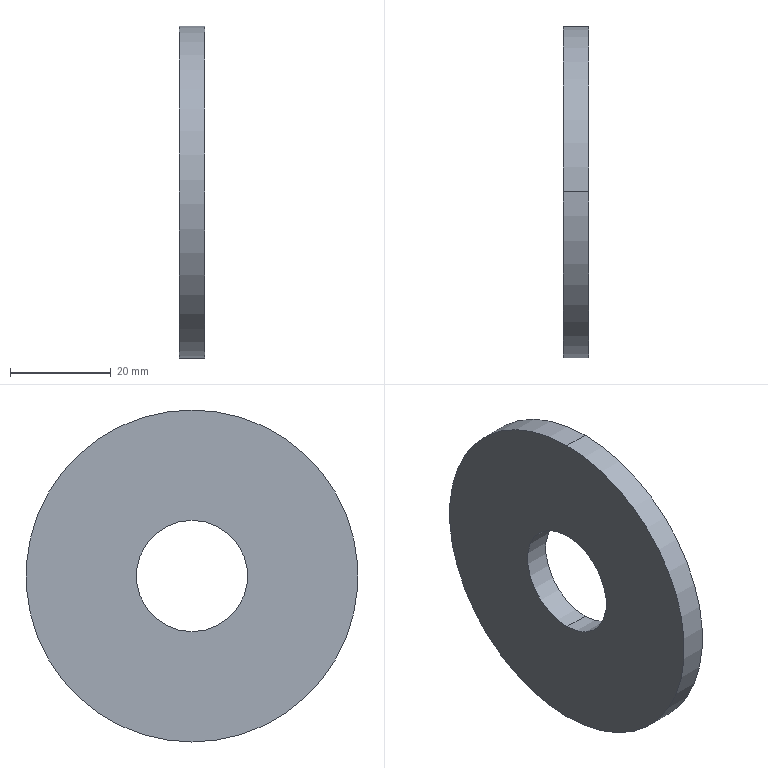Part | STEP file | flat washer wide_am_B18.22M - Plain washer, 20 mm, wide | 1 solid | 6 faces | box 5.1 x 66 x 66 mm | volume 15486 mm3 | cylinder 4 | plane 2 | commonest cylinder face diameters 22.13 x2 66 x2
STEP:
#1=CARTESIAN_POINT('',(0.,0.,0.));
#2=DIRECTION('',(0.,0.,1.));
#3=DIRECTION('',(1.,0.,0.));
#4=AXIS2_PLACEMENT_3D('',#1,#2,#3);
#5=CARTESIAN_POINT('',(0.,0.,33.));
#6=VERTEX_POINT('',#5);
#7=CARTESIAN_POINT('',(0.,0.,-33.));
#8=VERTEX_POINT('',#7);
#9=CARTESIAN_POINT('',(0.,0.,0.));
#10=DIRECTION('',(-1.,0.,0.));
#11=DIRECTION('',(0.,0.,1.));
#12=AXIS2_PLACEMENT_3D('',#9,#10,#11);
#13=CIRCLE('',#12,33.);
#14=CARTESIAN_POINT('',(-34.925,0.,0.));
#15=DIRECTION('',(-1.,0.,0.));
#16=DIRECTION('',(0.,0.,1.));
#17=AXIS2_PLACEMENT_3D('',#14,#15,#16);
#18=CYLINDRICAL_SURFACE('',#17,33.);
#19=CARTESIAN_POINT('',(0.,-34.925));
#20=DIRECTION('',(1.,0.));
#21=VECTOR('',#20,1.);
#22=LINE('',#19,#21);
#23=(GEOMETRIC_REPRESENTATION_CONTEXT(2)PARAMETRIC_REPRESENTATION_CONTEXT()REPRESENTATION_CONTEXT('',''));
#24=DEFINITIONAL_REPRESENTATION('',(#22),#23);
#25=PCURVE('',#18,#24);
#26=CARTESIAN_POINT('',(0.,11.065,0.));
#27=DIRECTION('',(-1.,0.,0.));
#28=DIRECTION('',(0.,0.,1.));
#29=AXIS2_PLACEMENT_3D('',#26,#27,#28);
#30=PLANE('',#29);
#31=CARTESIAN_POINT('',(0.,-11.065));
#32=DIRECTION('',(1.,0.));
#33=AXIS2_PLACEMENT_2D('',#31,#32);
#34=CIRCLE('',#33,33.);
#35=(GEOMETRIC_REPRESENTATION_CONTEXT(2)PARAMETRIC_REPRESENTATION_CONTEXT()REPRESENTATION_CONTEXT('',''));
#36=DEFINITIONAL_REPRESENTATION('',(#34),#35);
#37=PCURVE('',#30,#36);
#38=SURFACE_CURVE('',#13,(#25,#37),.PCURVE_S1.);
#39=EDGE_CURVE('',#6,#8,#38,.T.);
#40=ORIENTED_EDGE('',*,*,#39,.T.);
#41=CARTESIAN_POINT('',(-5.1,0.,-33.));
#42=VERTEX_POINT('',#41);
#43=CARTESIAN_POINT('',(-34.925,0.,-33.));
#44=DIRECTION('',(-1.,0.,0.));
#45=VECTOR('',#44,1.);
#46=LINE('',#43,#45);
#47=CARTESIAN_POINT('',(3.142,0.));
#48=DIRECTION('',(0.,1.));
#49=VECTOR('',#48,1.);
#50=LINE('',#47,#49);
#51=(GEOMETRIC_REPRESENTATION_CONTEXT(2)PARAMETRIC_REPRESENTATION_CONTEXT()REPRESENTATION_CONTEXT('',''));
#52=DEFINITIONAL_REPRESENTATION('',(#50),#51);
#53=PCURVE('',#18,#52);
#54=CARTESIAN_POINT('',(-34.925,0.,0.));
#55=DIRECTION('',(-1.,0.,0.));
#56=DIRECTION('',(0.,0.,1.));
#57=AXIS2_PLACEMENT_3D('',#54,#55,#56);
#58=CYLINDRICAL_SURFACE('',#57,33.);
#59=CARTESIAN_POINT('',(3.142,0.));
#60=DIRECTION('',(0.,1.));
#61=VECTOR('',#60,1.);
#62=LINE('',#59,#61);
#63=(GEOMETRIC_REPRESENTATION_CONTEXT(2)PARAMETRIC_REPRESENTATION_CONTEXT()REPRESENTATION_CONTEXT('',''));
#64=DEFINITIONAL_REPRESENTATION('',(#62),#63);
#65=PCURVE('',#58,#64);
#66=SURFACE_CURVE('',#46,(#53,#65),.PCURVE_S1.);
#67=EDGE_CURVE('',#8,#42,#66,.T.);
#68=ORIENTED_EDGE('',*,*,#67,.T.);
#69=CARTESIAN_POINT('',(-5.1,0.,33.));
#70=VERTEX_POINT('',#69);
#71=CARTESIAN_POINT('',(-5.1,0.,0.));
#72=DIRECTION('',(-1.,0.,0.));
#73=DIRECTION('',(0.,0.,1.));
#74=AXIS2_PLACEMENT_3D('',#71,#72,#73);
#75=CIRCLE('',#74,33.);
#76=CARTESIAN_POINT('',(0.,-29.825));
#77=DIRECTION('',(1.,0.));
#78=VECTOR('',#77,1.);
#79=LINE('',#76,#78);
#80=(GEOMETRIC_REPRESENTATION_CONTEXT(2)PARAMETRIC_REPRESENTATION_CONTEXT()REPRESENTATION_CONTEXT('',''));
#81=DEFINITIONAL_REPRESENTATION('',(#79),#80);
#82=PCURVE('',#18,#81);
#83=CARTESIAN_POINT('',(-5.1,33.,0.));
#84=DIRECTION('',(1.,0.,0.));
#85=DIRECTION('',(0.,0.,-1.));
#86=AXIS2_PLACEMENT_3D('',#83,#84,#85);
#87=PLANE('',#86);
#88=CARTESIAN_POINT('',(-33.,-33.));
#89=CARTESIAN_POINT('',(-33.,24.158));
#90=CARTESIAN_POINT('',(16.5,-4.421));
#91=CARTESIAN_POINT('',(66.,-33.));
#92=CARTESIAN_POINT('',(16.5,-61.579));
#93=CARTESIAN_POINT('',(-33.,-90.158));
#94=CARTESIAN_POINT('',(-33.,-33.));
#95=(BOUNDED_CURVE()B_SPLINE_CURVE(2,(#88,#89,#90,#91,#92,#93,#94),.UNSPECIFIED.,.T.,.F.)B_SPLINE_CURVE_WITH_KNOTS((1,2,2,2,2,1),(-2.094,0.,2.094,4.189,6.283,8.378),.UNSPECIFIED.)CURVE()GEOMETRIC_REPRESENTATION_ITEM()RATIONAL_B_SPLINE_CURVE((1.,0.5,1.,0.5,1.,0.5,1.))REPRESENTATION_ITEM(''));
#96=(GEOMETRIC_REPRESENTATION_CONTEXT(2)PARAMETRIC_REPRESENTATION_CONTEXT()REPRESENTATION_CONTEXT('',''));
#97=DEFINITIONAL_REPRESENTATION('',(#95),#96);
#98=PCURVE('',#87,#97);
#99=SURFACE_CURVE('',#75,(#82,#98),.PCURVE_S1.);
#100=EDGE_CURVE('',#70,#42,#99,.T.);
#101=ORIENTED_EDGE('',*,*,#100,.F.);
#102=CARTESIAN_POINT('',(-34.925,0.,33.));
#103=DIRECTION('',(-1.,0.,0.));
#104=VECTOR('',#103,1.);
#105=LINE('',#102,#104);
#106=CARTESIAN_POINT('',(0.,0.));
#107=DIRECTION('',(0.,1.));
#108=VECTOR('',#107,1.);
#109=LINE('',#106,#108);
#110=(GEOMETRIC_REPRESENTATION_CONTEXT(2)PARAMETRIC_REPRESENTATION_CONTEXT()REPRESENTATION_CONTEXT('',''));
#111=DEFINITIONAL_REPRESENTATION('',(#109),#110);
#112=PCURVE('',#18,#111);
#113=CARTESIAN_POINT('',(6.283,0.));
#114=DIRECTION('',(0.,1.));
#115=VECTOR('',#114,1.);
#116=LINE('',#113,#115);
#117=(GEOMETRIC_REPRESENTATION_CONTEXT(2)PARAMETRIC_REPRESENTATION_CONTEXT()REPRESENTATION_CONTEXT('',''));
#118=DEFINITIONAL_REPRESENTATION('',(#116),#117);
#119=PCURVE('',#58,#118);
#120=SURFACE_CURVE('',#105,(#112,#119),.PCURVE_S1.);
#121=EDGE_CURVE('',#6,#70,#120,.T.);
#122=ORIENTED_EDGE('',*,*,#121,.F.);
#123=EDGE_LOOP('',(#40,#68,#101,#122));
#124=FACE_BOUND('',#123,.T.);
#125=ADVANCED_FACE('',(#124),#18,.T.);
#126=CARTESIAN_POINT('',(0.,0.,11.065));
#127=VERTEX_POINT('',#126);
#128=CARTESIAN_POINT('',(-5.1,0.,11.065));
#129=VERTEX_POINT('',#128);
#130=CARTESIAN_POINT('',(-34.925,0.,11.065));
#131=DIRECTION('',(-1.,0.,0.));
#132=VECTOR('',#131,1.);
#133=LINE('',#130,#132);
#134=CARTESIAN_POINT('',(-34.925,0.,0.));
#135=DIRECTION('',(-1.,0.,0.));
#136=DIRECTION('',(0.,0.,1.));
#137=AXIS2_PLACEMENT_3D('',#134,#135,#136);
#138=CYLINDRICAL_SURFACE('',#137,11.065);
#139=CARTESIAN_POINT('',(6.283,0.));
#140=DIRECTION('',(0.,1.));
#141=VECTOR('',#140,1.);
#142=LINE('',#139,#141);
#143=(GEOMETRIC_REPRESENTATION_CONTEXT(2)PARAMETRIC_REPRESENTATION_CONTEXT()REPRESENTATION_CONTEXT('',''));
#144=DEFINITIONAL_REPRESENTATION('',(#142),#143);
#145=PCURVE('',#138,#144);
#146=CARTESIAN_POINT('',(-34.925,0.,0.));
#147=DIRECTION('',(-1.,0.,0.));
#148=DIRECTION('',(0.,0.,1.));
#149=AXIS2_PLACEMENT_3D('',#146,#147,#148);
#150=CYLINDRICAL_SURFACE('',#149,11.065);
#151=CARTESIAN_POINT('',(0.,0.));
#152=DIRECTION('',(0.,1.));
#153=VECTOR('',#152,1.);
#154=LINE('',#151,#153);
#155=(GEOMETRIC_REPRESENTATION_CONTEXT(2)PARAMETRIC_REPRESENTATION_CONTEXT()REPRESENTATION_CONTEXT('',''));
#156=DEFINITIONAL_REPRESENTATION('',(#154),#155);
#157=PCURVE('',#150,#156);
#158=SURFACE_CURVE('',#133,(#145,#157),.PCURVE_S1.);
#159=EDGE_CURVE('',#127,#129,#158,.T.);
#160=ORIENTED_EDGE('',*,*,#159,.T.);
#161=CARTESIAN_POINT('',(-5.1,0.,-11.065));
#162=VERTEX_POINT('',#161);
#163=CARTESIAN_POINT('',(-5.1,0.,0.));
#164=DIRECTION('',(-1.,0.,0.));
#165=DIRECTION('',(0.,0.,1.));
#166=AXIS2_PLACEMENT_3D('',#163,#164,#165);
#167=CIRCLE('',#166,11.065);
#168=CARTESIAN_POINT('',(0.,-29.825));
#169=DIRECTION('',(1.,0.));
#170=VECTOR('',#169,1.);
#171=LINE('',#168,#170);
#172=(GEOMETRIC_REPRESENTATION_CONTEXT(2)PARAMETRIC_REPRESENTATION_CONTEXT()REPRESENTATION_CONTEXT('',''));
#173=DEFINITIONAL_REPRESENTATION('',(#171),#172);
#174=PCURVE('',#138,#173);
#175=CARTESIAN_POINT('',(-11.065,-33.));
#176=CARTESIAN_POINT('',(-11.065,-13.835));
#177=CARTESIAN_POINT('',(5.532,-23.417));
#178=CARTESIAN_POINT('',(22.13,-33.));
#179=CARTESIAN_POINT('',(5.532,-42.583));
#180=CARTESIAN_POINT('',(-11.065,-52.165));
#181=CARTESIAN_POINT('',(-11.065,-33.));
#182=(BOUNDED_CURVE()B_SPLINE_CURVE(2,(#175,#176,#177,#178,#179,#180,#181),.UNSPECIFIED.,.T.,.F.)B_SPLINE_CURVE_WITH_KNOTS((1,2,2,2,2,1),(-2.094,0.,2.094,4.189,6.283,8.378),.UNSPECIFIED.)CURVE()GEOMETRIC_REPRESENTATION_ITEM()RATIONAL_B_SPLINE_CURVE((1.,0.5,1.,0.5,1.,0.5,1.))REPRESENTATION_ITEM(''));
#183=(GEOMETRIC_REPRESENTATION_CONTEXT(2)PARAMETRIC_REPRESENTATION_CONTEXT()REPRESENTATION_CONTEXT('',''));
#184=DEFINITIONAL_REPRESENTATION('',(#182),#183);
#185=PCURVE('',#87,#184);
#186=SURFACE_CURVE('',#167,(#174,#185),.PCURVE_S1.);
#187=EDGE_CURVE('',#162,#129,#186,.T.);
#188=ORIENTED_EDGE('',*,*,#187,.F.);
#189=CARTESIAN_POINT('',(0.,0.,-11.065));
#190=VERTEX_POINT('',#189);
#191=CARTESIAN_POINT('',(-34.925,0.,-11.065));
#192=DIRECTION('',(-1.,0.,0.));
#193=VECTOR('',#192,1.);
#194=LINE('',#191,#193);
#195=CARTESIAN_POINT('',(3.142,0.));
#196=DIRECTION('',(0.,1.));
#197=VECTOR('',#196,1.);
#198=LINE('',#195,#197);
#199=(GEOMETRIC_REPRESENTATION_CONTEXT(2)PARAMETRIC_REPRESENTATION_CONTEXT()REPRESENTATION_CONTEXT('',''));
#200=DEFINITIONAL_REPRESENTATION('',(#198),#199);
#201=PCURVE('',#138,#200);
#202=CARTESIAN_POINT('',(3.142,0.));
#203=DIRECTION('',(0.,1.));
#204=VECTOR('',#203,1.);
#205=LINE('',#202,#204);
#206=(GEOMETRIC_REPRESENTATION_CONTEXT(2)PARAMETRIC_REPRESENTATION_CONTEXT()REPRESENTATION_CONTEXT('',''));
#207=DEFINITIONAL_REPRESENTATION('',(#205),#206);
#208=PCURVE('',#150,#207);
#209=SURFACE_CURVE('',#194,(#201,#208),.PCURVE_S1.);
#210=EDGE_CURVE('',#190,#162,#209,.T.);
#211=ORIENTED_EDGE('',*,*,#210,.F.);
#212=CARTESIAN_POINT('',(0.,0.,0.));
#213=DIRECTION('',(-1.,0.,0.));
#214=DIRECTION('',(0.,0.,1.));
#215=AXIS2_PLACEMENT_3D('',#212,#213,#214);
#216=CIRCLE('',#215,11.065);
#217=CARTESIAN_POINT('',(0.,-34.925));
#218=DIRECTION('',(1.,0.));
#219=VECTOR('',#218,1.);
#220=LINE('',#217,#219);
#221=(GEOMETRIC_REPRESENTATION_CONTEXT(2)PARAMETRIC_REPRESENTATION_CONTEXT()REPRESENTATION_CONTEXT('',''));
#222=DEFINITIONAL_REPRESENTATION('',(#220),#221);
#223=PCURVE('',#138,#222);
#224=CARTESIAN_POINT('',(0.,-11.065));
#225=DIRECTION('',(1.,0.));
#226=AXIS2_PLACEMENT_2D('',#224,#225);
#227=CIRCLE('',#226,11.065);
#228=(GEOMETRIC_REPRESENTATION_CONTEXT(2)PARAMETRIC_REPRESENTATION_CONTEXT()REPRESENTATION_CONTEXT('',''));
#229=DEFINITIONAL_REPRESENTATION('',(#227),#228);
#230=PCURVE('',#30,#229);
#231=SURFACE_CURVE('',#216,(#223,#230),.PCURVE_S1.);
#232=EDGE_CURVE('',#190,#127,#231,.T.);
#233=ORIENTED_EDGE('',*,*,#232,.T.);
#234=EDGE_LOOP('',(#160,#188,#211,#233));
#235=FACE_BOUND('',#234,.F.);
#236=ADVANCED_FACE('',(#235),#138,.F.);
#237=CARTESIAN_POINT('',(-5.1,0.,0.));
#238=DIRECTION('',(-1.,0.,0.));
#239=DIRECTION('',(0.,0.,1.));
#240=AXIS2_PLACEMENT_3D('',#237,#238,#239);
#241=CIRCLE('',#240,11.065);
#242=CARTESIAN_POINT('',(0.,-29.825));
#243=DIRECTION('',(1.,0.));
#244=VECTOR('',#243,1.);
#245=LINE('',#242,#244);
#246=(GEOMETRIC_REPRESENTATION_CONTEXT(2)PARAMETRIC_REPRESENTATION_CONTEXT()REPRESENTATION_CONTEXT('',''));
#247=DEFINITIONAL_REPRESENTATION('',(#245),#246);
#248=PCURVE('',#150,#247);
#249=CARTESIAN_POINT('',(-11.065,-33.));
#250=CARTESIAN_POINT('',(-11.065,-13.835));
#251=CARTESIAN_POINT('',(5.532,-23.417));
#252=CARTESIAN_POINT('',(22.13,-33.));
#253=CARTESIAN_POINT('',(5.532,-42.583));
#254=CARTESIAN_POINT('',(-11.065,-52.165));
#255=CARTESIAN_POINT('',(-11.065,-33.));
#256=(BOUNDED_CURVE()B_SPLINE_CURVE(2,(#249,#250,#251,#252,#253,#254,#255),.UNSPECIFIED.,.T.,.F.)B_SPLINE_CURVE_WITH_KNOTS((1,2,2,2,2,1),(-2.094,0.,2.094,4.189,6.283,8.378),.UNSPECIFIED.)CURVE()GEOMETRIC_REPRESENTATION_ITEM()RATIONAL_B_SPLINE_CURVE((1.,0.5,1.,0.5,1.,0.5,1.))REPRESENTATION_ITEM(''));
#257=(GEOMETRIC_REPRESENTATION_CONTEXT(2)PARAMETRIC_REPRESENTATION_CONTEXT()REPRESENTATION_CONTEXT('',''));
#258=DEFINITIONAL_REPRESENTATION('',(#256),#257);
#259=PCURVE('',#87,#258);
#260=SURFACE_CURVE('',#241,(#248,#259),.PCURVE_S1.);
#261=EDGE_CURVE('',#129,#162,#260,.T.);
#262=ORIENTED_EDGE('',*,*,#261,.F.);
#263=ORIENTED_EDGE('',*,*,#159,.F.);
#264=CARTESIAN_POINT('',(0.,0.,0.));
#265=DIRECTION('',(-1.,0.,0.));
#266=DIRECTION('',(0.,0.,1.));
#267=AXIS2_PLACEMENT_3D('',#264,#265,#266);
#268=CIRCLE('',#267,11.065);
#269=CARTESIAN_POINT('',(0.,-34.925));
#270=DIRECTION('',(1.,0.));
#271=VECTOR('',#270,1.);
#272=LINE('',#269,#271);
#273=(GEOMETRIC_REPRESENTATION_CONTEXT(2)PARAMETRIC_REPRESENTATION_CONTEXT()REPRESENTATION_CONTEXT('',''));
#274=DEFINITIONAL_REPRESENTATION('',(#272),#273);
#275=PCURVE('',#150,#274);
#276=CARTESIAN_POINT('',(0.,-11.065));
#277=DIRECTION('',(1.,0.));
#278=AXIS2_PLACEMENT_2D('',#276,#277);
#279=CIRCLE('',#278,11.065);
#280=(GEOMETRIC_REPRESENTATION_CONTEXT(2)PARAMETRIC_REPRESENTATION_CONTEXT()REPRESENTATION_CONTEXT('',''));
#281=DEFINITIONAL_REPRESENTATION('',(#279),#280);
#282=PCURVE('',#30,#281);
#283=SURFACE_CURVE('',#268,(#275,#282),.PCURVE_S1.);
#284=EDGE_CURVE('',#127,#190,#283,.T.);
#285=ORIENTED_EDGE('',*,*,#284,.T.);
#286=ORIENTED_EDGE('',*,*,#210,.T.);
#287=EDGE_LOOP('',(#262,#263,#285,#286));
#288=FACE_BOUND('',#287,.F.);
#289=ADVANCED_FACE('',(#288),#150,.F.);
#290=ORIENTED_EDGE('',*,*,#39,.F.);
#291=CARTESIAN_POINT('',(0.,0.,0.));
#292=DIRECTION('',(-1.,0.,0.));
#293=DIRECTION('',(0.,0.,1.));
#294=AXIS2_PLACEMENT_3D('',#291,#292,#293);
#295=CIRCLE('',#294,33.);
#296=CARTESIAN_POINT('',(0.,-11.065));
#297=DIRECTION('',(1.,0.));
#298=AXIS2_PLACEMENT_2D('',#296,#297);
#299=CIRCLE('',#298,33.);
#300=(GEOMETRIC_REPRESENTATION_CONTEXT(2)PARAMETRIC_REPRESENTATION_CONTEXT()REPRESENTATION_CONTEXT('',''));
#301=DEFINITIONAL_REPRESENTATION('',(#299),#300);
#302=PCURVE('',#30,#301);
#303=CARTESIAN_POINT('',(0.,-34.925));
#304=DIRECTION('',(1.,0.));
#305=VECTOR('',#304,1.);
#306=LINE('',#303,#305);
#307=(GEOMETRIC_REPRESENTATION_CONTEXT(2)PARAMETRIC_REPRESENTATION_CONTEXT()REPRESENTATION_CONTEXT('',''));
#308=DEFINITIONAL_REPRESENTATION('',(#306),#307);
#309=PCURVE('',#58,#308);
#310=SURFACE_CURVE('',#295,(#302,#309),.PCURVE_S1.);
#311=EDGE_CURVE('',#8,#6,#310,.T.);
#312=ORIENTED_EDGE('',*,*,#311,.F.);
#313=EDGE_LOOP('',(#290,#312));
#314=FACE_BOUND('',#313,.T.);
#315=ORIENTED_EDGE('',*,*,#284,.T.);
#316=ORIENTED_EDGE('',*,*,#232,.T.);
#317=EDGE_LOOP('',(#315,#316));
#318=FACE_BOUND('',#317,.T.);
#319=ADVANCED_FACE('',(#314,#318),#30,.F.);
#320=ORIENTED_EDGE('',*,*,#67,.F.);
#321=ORIENTED_EDGE('',*,*,#311,.T.);
#322=ORIENTED_EDGE('',*,*,#121,.T.);
#323=CARTESIAN_POINT('',(-5.1,0.,0.));
#324=DIRECTION('',(-1.,0.,0.));
#325=DIRECTION('',(0.,0.,1.));
#326=AXIS2_PLACEMENT_3D('',#323,#324,#325);
#327=CIRCLE('',#326,33.);
#328=CARTESIAN_POINT('',(0.,-29.825));
#329=DIRECTION('',(1.,0.));
#330=VECTOR('',#329,1.);
#331=LINE('',#328,#330);
#332=(GEOMETRIC_REPRESENTATION_CONTEXT(2)PARAMETRIC_REPRESENTATION_CONTEXT()REPRESENTATION_CONTEXT('',''));
#333=DEFINITIONAL_REPRESENTATION('',(#331),#332);
#334=PCURVE('',#58,#333);
#335=CARTESIAN_POINT('',(-33.,-33.));
#336=CARTESIAN_POINT('',(-33.,24.158));
#337=CARTESIAN_POINT('',(16.5,-4.421));
#338=CARTESIAN_POINT('',(66.,-33.));
#339=CARTESIAN_POINT('',(16.5,-61.579));
#340=CARTESIAN_POINT('',(-33.,-90.158));
#341=CARTESIAN_POINT('',(-33.,-33.));
#342=(BOUNDED_CURVE()B_SPLINE_CURVE(2,(#335,#336,#337,#338,#339,#340,#341),.UNSPECIFIED.,.T.,.F.)B_SPLINE_CURVE_WITH_KNOTS((1,2,2,2,2,1),(-2.094,0.,2.094,4.189,6.283,8.378),.UNSPECIFIED.)CURVE()GEOMETRIC_REPRESENTATION_ITEM()RATIONAL_B_SPLINE_CURVE((1.,0.5,1.,0.5,1.,0.5,1.))REPRESENTATION_ITEM(''));
#343=(GEOMETRIC_REPRESENTATION_CONTEXT(2)PARAMETRIC_REPRESENTATION_CONTEXT()REPRESENTATION_CONTEXT('',''));
#344=DEFINITIONAL_REPRESENTATION('',(#342),#343);
#345=PCURVE('',#87,#344);
#346=SURFACE_CURVE('',#327,(#334,#345),.PCURVE_S1.);
#347=EDGE_CURVE('',#42,#70,#346,.T.);
#348=ORIENTED_EDGE('',*,*,#347,.F.);
#349=EDGE_LOOP('',(#320,#321,#322,#348));
#350=FACE_BOUND('',#349,.T.);
#351=ADVANCED_FACE('',(#350),#58,.T.);
#352=ORIENTED_EDGE('',*,*,#261,.F.);
#353=ORIENTED_EDGE('',*,*,#187,.F.);
#354=EDGE_LOOP('',(#352,#353));
#355=FACE_BOUND('',#354,.T.);
#356=ORIENTED_EDGE('',*,*,#100,.T.);
#357=ORIENTED_EDGE('',*,*,#347,.T.);
#358=EDGE_LOOP('',(#356,#357));
#359=FACE_BOUND('',#358,.T.);
#360=ADVANCED_FACE('',(#355,#359),#87,.F.);
#361=CLOSED_SHELL('',(#125,#236,#289,#319,#351,#360));
#362=MANIFOLD_SOLID_BREP('',#361);
#363=(LENGTH_UNIT()NAMED_UNIT(*)SI_UNIT(.MILLI.,.METRE.));
#364=UNCERTAINTY_MEASURE_WITH_UNIT(LENGTH_MEASURE(0.0000001),#363,'','');
#365=(NAMED_UNIT(*)PLANE_ANGLE_UNIT()SI_UNIT($,.RADIAN.));
#366=(NAMED_UNIT(*)SI_UNIT($,.STERADIAN.)SOLID_ANGLE_UNIT());
#367=(GEOMETRIC_REPRESENTATION_CONTEXT(3)GLOBAL_UNCERTAINTY_ASSIGNED_CONTEXT((#364))GLOBAL_UNIT_ASSIGNED_CONTEXT((#363,#365,#366))REPRESENTATION_CONTEXT('',''));
#368=ADVANCED_BREP_SHAPE_REPRESENTATION('',(#4,#362),#367);